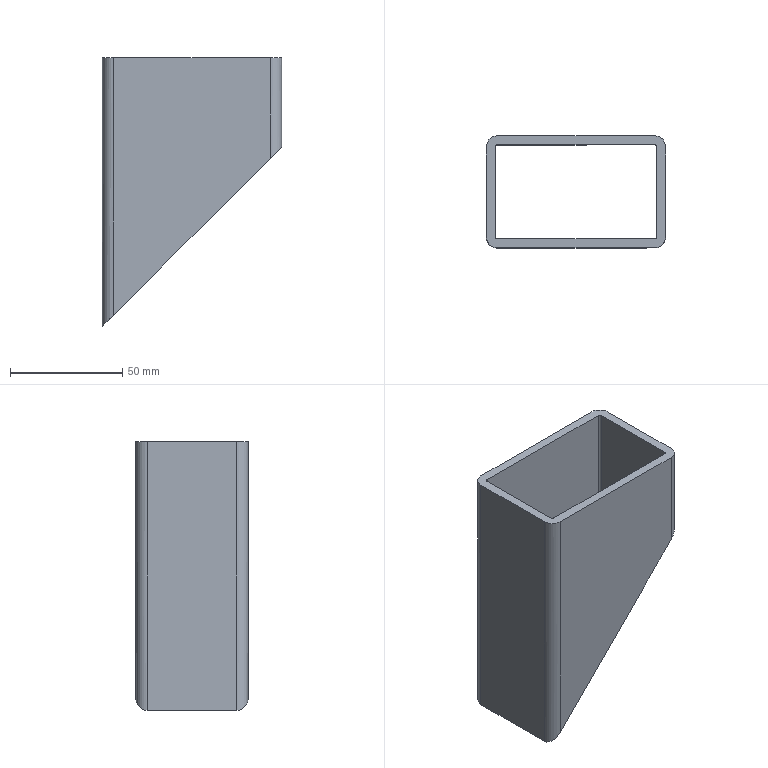Part | SolidWorks | features ICE 3, Extrusion 1, Shell 1 | 1 solid | 18 faces | box 80 x 50 x 120 mm | volume 76432 mm3 | plane 10 | cylinder 8 | commonest cylinder face diameters 2 x4 10 x4
STEP:
#1=CARTESIAN_POINT('',(-40.,20.,120.));
#2=VERTEX_POINT('',#1);
#3=CARTESIAN_POINT('',(-40.,20.,0.));
#4=VERTEX_POINT('',#3);
#5=CARTESIAN_POINT('',(-40.,20.,2200.));
#6=DIRECTION('',(0.,0.,-1.));
#7=VECTOR('',#6,1000.);
#8=LINE('',#5,#7);
#9=EDGE_CURVE('',#2,#4,#8,.T.);
#10=ORIENTED_EDGE('',*,*,#9,.F.);
#11=CARTESIAN_POINT('',(-35.,25.,120.));
#12=VERTEX_POINT('',#11);
#13=CARTESIAN_POINT('',(-35.,20.,120.));
#14=DIRECTION('',(0.,0.,-1.));
#15=DIRECTION('',(-1.,0.,0.));
#16=AXIS2_PLACEMENT_3D('',#13,#14,#15);
#17=CIRCLE('',#16,5.);
#18=EDGE_CURVE('',#2,#12,#17,.T.);
#19=ORIENTED_EDGE('',*,*,#18,.T.);
#20=CARTESIAN_POINT('',(-35.,25.,5.));
#21=VERTEX_POINT('',#20);
#22=CARTESIAN_POINT('',(-35.,25.,2200.));
#23=DIRECTION('',(0.,0.,-1.));
#24=VECTOR('',#23,1000.);
#25=LINE('',#22,#24);
#26=EDGE_CURVE('',#12,#21,#25,.T.);
#27=ORIENTED_EDGE('',*,*,#26,.T.);
#28=CARTESIAN_POINT('',(-35.,25.,5.));
#29=CARTESIAN_POINT('',(-37.929,25.,2.071));
#30=CARTESIAN_POINT('',(-40.,22.929,0.));
#31=CARTESIAN_POINT('',(-40.,20.,0.));
#32=(BOUNDED_CURVE()B_SPLINE_CURVE(3,(#28,#29,#30,#31),.UNSPECIFIED.,.F.,.T.)B_SPLINE_CURVE_WITH_KNOTS((4,4),(4.712,6.283),.UNSPECIFIED.)CURVE()GEOMETRIC_REPRESENTATION_ITEM()RATIONAL_B_SPLINE_CURVE((1.,0.8047,0.8047,1.))REPRESENTATION_ITEM(''));
#33=EDGE_CURVE('',#21,#4,#32,.T.);
#34=ORIENTED_EDGE('',*,*,#33,.T.);
#35=EDGE_LOOP('',(#10,#19,#27,#34));
#36=FACE_OUTER_BOUND('',#35,.T.);
#37=CARTESIAN_POINT('',(-35.,20.,2200.));
#38=DIRECTION('',(0.,0.,-1.));
#39=DIRECTION('',(-1.,0.,0.));
#40=AXIS2_PLACEMENT_3D('',#37,#38,#39);
#41=CYLINDRICAL_SURFACE('',#40,5.);
#42=ADVANCED_FACE('',(#36),#41,.T.);
#43=CARTESIAN_POINT('',(-40.,-20.,120.));
#44=VERTEX_POINT('',#43);
#45=CARTESIAN_POINT('',(-40.,-20.,0.));
#46=VERTEX_POINT('',#45);
#47=CARTESIAN_POINT('',(-40.,-20.,2200.));
#48=DIRECTION('',(0.,0.,-1.));
#49=VECTOR('',#48,1000.);
#50=LINE('',#47,#49);
#51=EDGE_CURVE('',#44,#46,#50,.T.);
#52=ORIENTED_EDGE('',*,*,#51,.F.);
#53=CARTESIAN_POINT('',(-40.,20.,120.));
#54=DIRECTION('',(0.,1.,0.));
#55=VECTOR('',#54,1000.);
#56=LINE('',#53,#55);
#57=EDGE_CURVE('',#44,#2,#56,.T.);
#58=ORIENTED_EDGE('',*,*,#57,.T.);
#59=ORIENTED_EDGE('',*,*,#9,.T.);
#60=CARTESIAN_POINT('',(-40.,20.,0.));
#61=DIRECTION('',(0.,-1.,0.));
#62=VECTOR('',#61,1000.);
#63=LINE('',#60,#62);
#64=EDGE_CURVE('',#4,#46,#63,.T.);
#65=ORIENTED_EDGE('',*,*,#64,.T.);
#66=EDGE_LOOP('',(#52,#58,#59,#65));
#67=FACE_OUTER_BOUND('',#66,.T.);
#68=CARTESIAN_POINT('',(-40.,20.,2200.));
#69=DIRECTION('',(1.,0.,0.));
#70=DIRECTION('',(0.,1.,0.));
#71=AXIS2_PLACEMENT_3D('',#68,#69,#70);
#72=PLANE('',#71);
#73=ADVANCED_FACE('',(#67),#72,.F.);
#74=CARTESIAN_POINT('',(-35.,-25.,120.));
#75=VERTEX_POINT('',#74);
#76=CARTESIAN_POINT('',(-35.,-20.,120.));
#77=DIRECTION('',(0.,0.,1.));
#78=DIRECTION('',(-1.,0.,0.));
#79=AXIS2_PLACEMENT_3D('',#76,#77,#78);
#80=CIRCLE('',#79,5.);
#81=EDGE_CURVE('',#44,#75,#80,.T.);
#82=ORIENTED_EDGE('',*,*,#81,.F.);
#83=ORIENTED_EDGE('',*,*,#51,.T.);
#84=CARTESIAN_POINT('',(-35.,-25.,5.));
#85=VERTEX_POINT('',#84);
#86=CARTESIAN_POINT('',(-35.,-25.,5.));
#87=CARTESIAN_POINT('',(-37.929,-25.,2.071));
#88=CARTESIAN_POINT('',(-40.,-22.929,0.));
#89=CARTESIAN_POINT('',(-40.,-20.,0.));
#90=(BOUNDED_CURVE()B_SPLINE_CURVE(3,(#86,#87,#88,#89),.UNSPECIFIED.,.F.,.F.)B_SPLINE_CURVE_WITH_KNOTS((4,4),(4.712,6.283),.UNSPECIFIED.)CURVE()GEOMETRIC_REPRESENTATION_ITEM()RATIONAL_B_SPLINE_CURVE((1.,0.8047,0.8047,1.))REPRESENTATION_ITEM(''));
#91=EDGE_CURVE('',#85,#46,#90,.T.);
#92=ORIENTED_EDGE('',*,*,#91,.F.);
#93=CARTESIAN_POINT('',(-35.,-25.,2200.));
#94=DIRECTION('',(0.,0.,-1.));
#95=VECTOR('',#94,1000.);
#96=LINE('',#93,#95);
#97=EDGE_CURVE('',#75,#85,#96,.T.);
#98=ORIENTED_EDGE('',*,*,#97,.F.);
#99=EDGE_LOOP('',(#82,#83,#92,#98));
#100=FACE_OUTER_BOUND('',#99,.T.);
#101=CARTESIAN_POINT('',(-35.,-20.,2200.));
#102=DIRECTION('',(0.,0.,-1.));
#103=DIRECTION('',(-1.,0.,0.));
#104=AXIS2_PLACEMENT_3D('',#101,#102,#103);
#105=CYLINDRICAL_SURFACE('',#104,5.);
#106=ADVANCED_FACE('',(#100),#105,.T.);
#107=CARTESIAN_POINT('',(35.,-25.,120.));
#108=VERTEX_POINT('',#107);
#109=CARTESIAN_POINT('',(1017.702,-25.,120.));
#110=DIRECTION('',(1.,0.,0.));
#111=VECTOR('',#110,1000.);
#112=LINE('',#109,#111);
#113=EDGE_CURVE('',#75,#108,#112,.T.);
#114=ORIENTED_EDGE('',*,*,#113,.F.);
#115=ORIENTED_EDGE('',*,*,#97,.T.);
#116=CARTESIAN_POINT('',(35.,-25.,75.));
#117=VERTEX_POINT('',#116);
#118=CARTESIAN_POINT('',(-40.,-25.,0.));
#119=DIRECTION('',(-0.7071,0.,-0.7071));
#120=VECTOR('',#119,1000.);
#121=LINE('',#118,#120);
#122=EDGE_CURVE('',#117,#85,#121,.T.);
#123=ORIENTED_EDGE('',*,*,#122,.F.);
#124=CARTESIAN_POINT('',(35.,-25.,2200.));
#125=DIRECTION('',(0.,0.,-1.));
#126=VECTOR('',#125,1000.);
#127=LINE('',#124,#126);
#128=EDGE_CURVE('',#108,#117,#127,.T.);
#129=ORIENTED_EDGE('',*,*,#128,.F.);
#130=EDGE_LOOP('',(#114,#115,#123,#129));
#131=FACE_OUTER_BOUND('',#130,.T.);
#132=CARTESIAN_POINT('',(35.,-25.,2200.));
#133=DIRECTION('',(0.,-1.,0.));
#134=DIRECTION('',(1.,0.,0.));
#135=AXIS2_PLACEMENT_3D('',#132,#133,#134);
#136=PLANE('',#135);
#137=ADVANCED_FACE('',(#131),#136,.T.);
#138=CARTESIAN_POINT('',(40.,-20.,120.));
#139=VERTEX_POINT('',#138);
#140=CARTESIAN_POINT('',(35.,-20.,120.));
#141=DIRECTION('',(0.,0.,1.));
#142=DIRECTION('',(-1.,0.,0.));
#143=AXIS2_PLACEMENT_3D('',#140,#141,#142);
#144=CIRCLE('',#143,5.);
#145=EDGE_CURVE('',#108,#139,#144,.T.);
#146=ORIENTED_EDGE('',*,*,#145,.F.);
#147=ORIENTED_EDGE('',*,*,#128,.T.);
#148=CARTESIAN_POINT('',(40.,-20.,80.));
#149=VERTEX_POINT('',#148);
#150=CARTESIAN_POINT('',(40.,-20.,80.));
#151=CARTESIAN_POINT('',(40.,-22.929,80.));
#152=CARTESIAN_POINT('',(37.929,-25.,77.929));
#153=CARTESIAN_POINT('',(35.,-25.,75.));
#154=(BOUNDED_CURVE()B_SPLINE_CURVE(3,(#150,#151,#152,#153),.UNSPECIFIED.,.F.,.F.)B_SPLINE_CURVE_WITH_KNOTS((4,4),(3.142,4.712),.UNSPECIFIED.)CURVE()GEOMETRIC_REPRESENTATION_ITEM()RATIONAL_B_SPLINE_CURVE((1.,0.8047,0.8047,1.))REPRESENTATION_ITEM(''));
#155=EDGE_CURVE('',#149,#117,#154,.T.);
#156=ORIENTED_EDGE('',*,*,#155,.F.);
#157=CARTESIAN_POINT('',(40.,-20.,2200.));
#158=DIRECTION('',(0.,0.,-1.));
#159=VECTOR('',#158,1000.);
#160=LINE('',#157,#159);
#161=EDGE_CURVE('',#139,#149,#160,.T.);
#162=ORIENTED_EDGE('',*,*,#161,.F.);
#163=EDGE_LOOP('',(#146,#147,#156,#162));
#164=FACE_OUTER_BOUND('',#163,.T.);
#165=CARTESIAN_POINT('',(35.,-20.,2200.));
#166=DIRECTION('',(0.,0.,-1.));
#167=DIRECTION('',(-1.,0.,0.));
#168=AXIS2_PLACEMENT_3D('',#165,#166,#167);
#169=CYLINDRICAL_SURFACE('',#168,5.);
#170=ADVANCED_FACE('',(#164),#169,.T.);
#171=CARTESIAN_POINT('',(40.,20.,120.));
#172=VERTEX_POINT('',#171);
#173=CARTESIAN_POINT('',(40.,20.,120.));
#174=DIRECTION('',(0.,1.,0.));
#175=VECTOR('',#174,1000.);
#176=LINE('',#173,#175);
#177=EDGE_CURVE('',#139,#172,#176,.T.);
#178=ORIENTED_EDGE('',*,*,#177,.F.);
#179=ORIENTED_EDGE('',*,*,#161,.T.);
#180=CARTESIAN_POINT('',(40.,20.,80.));
#181=VERTEX_POINT('',#180);
#182=CARTESIAN_POINT('',(40.,1975.,80.));
#183=DIRECTION('',(0.,-1.,0.));
#184=VECTOR('',#183,1000.);
#185=LINE('',#182,#184);
#186=EDGE_CURVE('',#181,#149,#185,.T.);
#187=ORIENTED_EDGE('',*,*,#186,.F.);
#188=CARTESIAN_POINT('',(40.,20.,2200.));
#189=DIRECTION('',(0.,0.,-1.));
#190=VECTOR('',#189,1000.);
#191=LINE('',#188,#190);
#192=EDGE_CURVE('',#172,#181,#191,.T.);
#193=ORIENTED_EDGE('',*,*,#192,.F.);
#194=EDGE_LOOP('',(#178,#179,#187,#193));
#195=FACE_OUTER_BOUND('',#194,.T.);
#196=CARTESIAN_POINT('',(40.,20.,2200.));
#197=DIRECTION('',(1.,0.,0.));
#198=DIRECTION('',(0.,1.,0.));
#199=AXIS2_PLACEMENT_3D('',#196,#197,#198);
#200=PLANE('',#199);
#201=ADVANCED_FACE('',(#195),#200,.T.);
#202=CARTESIAN_POINT('',(35.,25.,120.));
#203=VERTEX_POINT('',#202);
#204=CARTESIAN_POINT('',(35.,20.,120.));
#205=DIRECTION('',(0.,0.,1.));
#206=DIRECTION('',(-1.,0.,0.));
#207=AXIS2_PLACEMENT_3D('',#204,#205,#206);
#208=CIRCLE('',#207,5.);
#209=EDGE_CURVE('',#172,#203,#208,.T.);
#210=ORIENTED_EDGE('',*,*,#209,.F.);
#211=ORIENTED_EDGE('',*,*,#192,.T.);
#212=CARTESIAN_POINT('',(35.,25.,75.));
#213=VERTEX_POINT('',#212);
#214=CARTESIAN_POINT('',(35.,25.,75.));
#215=CARTESIAN_POINT('',(37.929,25.,77.929));
#216=CARTESIAN_POINT('',(40.,22.929,80.));
#217=CARTESIAN_POINT('',(40.,20.,80.));
#218=(BOUNDED_CURVE()B_SPLINE_CURVE(3,(#214,#215,#216,#217),.UNSPECIFIED.,.F.,.F.)B_SPLINE_CURVE_WITH_KNOTS((4,4),(1.571,3.142),.UNSPECIFIED.)CURVE()GEOMETRIC_REPRESENTATION_ITEM()RATIONAL_B_SPLINE_CURVE((1.,0.8047,0.8047,1.))REPRESENTATION_ITEM(''));
#219=EDGE_CURVE('',#213,#181,#218,.T.);
#220=ORIENTED_EDGE('',*,*,#219,.F.);
#221=CARTESIAN_POINT('',(35.,25.,2200.));
#222=DIRECTION('',(0.,0.,-1.));
#223=VECTOR('',#222,1000.);
#224=LINE('',#221,#223);
#225=EDGE_CURVE('',#203,#213,#224,.T.);
#226=ORIENTED_EDGE('',*,*,#225,.F.);
#227=EDGE_LOOP('',(#210,#211,#220,#226));
#228=FACE_OUTER_BOUND('',#227,.T.);
#229=CARTESIAN_POINT('',(35.,20.,2200.));
#230=DIRECTION('',(0.,0.,-1.));
#231=DIRECTION('',(-1.,0.,0.));
#232=AXIS2_PLACEMENT_3D('',#229,#230,#231);
#233=CYLINDRICAL_SURFACE('',#232,5.);
#234=ADVANCED_FACE('',(#228),#233,.T.);
#235=ORIENTED_EDGE('',*,*,#26,.F.);
#236=CARTESIAN_POINT('',(35.,25.,120.));
#237=DIRECTION('',(1.,0.,0.));
#238=VECTOR('',#237,1000.);
#239=LINE('',#236,#238);
#240=EDGE_CURVE('',#12,#203,#239,.T.);
#241=ORIENTED_EDGE('',*,*,#240,.T.);
#242=ORIENTED_EDGE('',*,*,#225,.T.);
#243=CARTESIAN_POINT('',(1097.5,25.,1137.5));
#244=DIRECTION('',(-0.7071,0.,-0.7071));
#245=VECTOR('',#244,1000.);
#246=LINE('',#243,#245);
#247=EDGE_CURVE('',#213,#21,#246,.T.);
#248=ORIENTED_EDGE('',*,*,#247,.T.);
#249=EDGE_LOOP('',(#235,#241,#242,#248));
#250=FACE_OUTER_BOUND('',#249,.T.);
#251=CARTESIAN_POINT('',(35.,25.,2200.));
#252=DIRECTION('',(0.,-1.,0.));
#253=DIRECTION('',(1.,0.,0.));
#254=AXIS2_PLACEMENT_3D('',#251,#252,#253);
#255=PLANE('',#254);
#256=ADVANCED_FACE('',(#250),#255,.F.);
#257=CARTESIAN_POINT('',(-36.,20.,120.));
#258=VERTEX_POINT('',#257);
#259=CARTESIAN_POINT('',(-35.,21.,120.));
#260=VERTEX_POINT('',#259);
#261=CARTESIAN_POINT('',(-35.,20.,120.));
#262=DIRECTION('',(0.,0.,-1.));
#263=DIRECTION('',(-1.,0.,0.));
#264=AXIS2_PLACEMENT_3D('',#261,#262,#263);
#265=CIRCLE('',#264,1.);
#266=EDGE_CURVE('',#258,#260,#265,.T.);
#267=ORIENTED_EDGE('',*,*,#266,.F.);
#268=CARTESIAN_POINT('',(-36.,20.,4.));
#269=VERTEX_POINT('',#268);
#270=CARTESIAN_POINT('',(-36.,20.,2200.));
#271=DIRECTION('',(0.,0.,-1.));
#272=VECTOR('',#271,1000.);
#273=LINE('',#270,#272);
#274=EDGE_CURVE('',#258,#269,#273,.T.);
#275=ORIENTED_EDGE('',*,*,#274,.T.);
#276=CARTESIAN_POINT('',(-35.,21.,5.));
#277=VERTEX_POINT('',#276);
#278=CARTESIAN_POINT('',(-35.,21.,5.));
#279=CARTESIAN_POINT('',(-35.586,21.,4.414));
#280=CARTESIAN_POINT('',(-36.,20.586,4.));
#281=CARTESIAN_POINT('',(-36.,20.,4.));
#282=(BOUNDED_CURVE()B_SPLINE_CURVE(3,(#278,#279,#280,#281),.UNSPECIFIED.,.F.,.T.)B_SPLINE_CURVE_WITH_KNOTS((4,4),(4.712,6.283),.UNSPECIFIED.)CURVE()GEOMETRIC_REPRESENTATION_ITEM()RATIONAL_B_SPLINE_CURVE((1.,0.8047,0.8047,1.))REPRESENTATION_ITEM(''));
#283=EDGE_CURVE('',#277,#269,#282,.T.);
#284=ORIENTED_EDGE('',*,*,#283,.F.);
#285=CARTESIAN_POINT('',(-35.,21.,2200.));
#286=DIRECTION('',(0.,0.,-1.));
#287=VECTOR('',#286,1000.);
#288=LINE('',#285,#287);
#289=EDGE_CURVE('',#260,#277,#288,.T.);
#290=ORIENTED_EDGE('',*,*,#289,.F.);
#291=EDGE_LOOP('',(#267,#275,#284,#290));
#292=FACE_OUTER_BOUND('',#291,.T.);
#293=CARTESIAN_POINT('',(-35.,20.,2200.));
#294=DIRECTION('',(0.,0.,-1.));
#295=DIRECTION('',(-1.,0.,0.));
#296=AXIS2_PLACEMENT_3D('',#293,#294,#295);
#297=CYLINDRICAL_SURFACE('',#296,1.);
#298=ADVANCED_FACE('',(#292),#297,.F.);
#299=CARTESIAN_POINT('',(-36.,-20.,120.));
#300=VERTEX_POINT('',#299);
#301=CARTESIAN_POINT('',(-36.,20.,120.));
#302=DIRECTION('',(0.,1.,0.));
#303=VECTOR('',#302,1000.);
#304=LINE('',#301,#303);
#305=EDGE_CURVE('',#300,#258,#304,.T.);
#306=ORIENTED_EDGE('',*,*,#305,.F.);
#307=CARTESIAN_POINT('',(-36.,-20.,4.));
#308=VERTEX_POINT('',#307);
#309=CARTESIAN_POINT('',(-36.,-20.,2200.));
#310=DIRECTION('',(0.,0.,-1.));
#311=VECTOR('',#310,1000.);
#312=LINE('',#309,#311);
#313=EDGE_CURVE('',#300,#308,#312,.T.);
#314=ORIENTED_EDGE('',*,*,#313,.T.);
#315=CARTESIAN_POINT('',(-36.,20.,4.));
#316=DIRECTION('',(0.,-1.,0.));
#317=VECTOR('',#316,1000.);
#318=LINE('',#315,#317);
#319=EDGE_CURVE('',#269,#308,#318,.T.);
#320=ORIENTED_EDGE('',*,*,#319,.F.);
#321=ORIENTED_EDGE('',*,*,#274,.F.);
#322=EDGE_LOOP('',(#306,#314,#320,#321));
#323=FACE_OUTER_BOUND('',#322,.T.);
#324=CARTESIAN_POINT('',(-36.,20.,2200.));
#325=DIRECTION('',(1.,0.,0.));
#326=DIRECTION('',(0.,1.,0.));
#327=AXIS2_PLACEMENT_3D('',#324,#325,#326);
#328=PLANE('',#327);
#329=ADVANCED_FACE('',(#323),#328,.T.);
#330=ORIENTED_EDGE('',*,*,#313,.F.);
#331=CARTESIAN_POINT('',(-35.,-21.,120.));
#332=VERTEX_POINT('',#331);
#333=CARTESIAN_POINT('',(-35.,-20.,120.));
#334=DIRECTION('',(0.,0.,1.));
#335=DIRECTION('',(-1.,0.,0.));
#336=AXIS2_PLACEMENT_3D('',#333,#334,#335);
#337=CIRCLE('',#336,1.);
#338=EDGE_CURVE('',#300,#332,#337,.T.);
#339=ORIENTED_EDGE('',*,*,#338,.T.);
#340=CARTESIAN_POINT('',(-35.,-21.,5.));
#341=VERTEX_POINT('',#340);
#342=CARTESIAN_POINT('',(-35.,-21.,2200.));
#343=DIRECTION('',(0.,0.,-1.));
#344=VECTOR('',#343,1000.);
#345=LINE('',#342,#344);
#346=EDGE_CURVE('',#332,#341,#345,.T.);
#347=ORIENTED_EDGE('',*,*,#346,.T.);
#348=CARTESIAN_POINT('',(-35.,-21.,5.));
#349=CARTESIAN_POINT('',(-35.586,-21.,4.414));
#350=CARTESIAN_POINT('',(-36.,-20.586,4.));
#351=CARTESIAN_POINT('',(-36.,-20.,4.));
#352=(BOUNDED_CURVE()B_SPLINE_CURVE(3,(#348,#349,#350,#351),.UNSPECIFIED.,.F.,.F.)B_SPLINE_CURVE_WITH_KNOTS((4,4),(4.712,6.283),.UNSPECIFIED.)CURVE()GEOMETRIC_REPRESENTATION_ITEM()RATIONAL_B_SPLINE_CURVE((1.,0.8047,0.8047,1.))REPRESENTATION_ITEM(''));
#353=EDGE_CURVE('',#341,#308,#352,.T.);
#354=ORIENTED_EDGE('',*,*,#353,.T.);
#355=EDGE_LOOP('',(#330,#339,#347,#354));
#356=FACE_OUTER_BOUND('',#355,.T.);
#357=CARTESIAN_POINT('',(-35.,-20.,2200.));
#358=DIRECTION('',(0.,0.,-1.));
#359=DIRECTION('',(-1.,0.,0.));
#360=AXIS2_PLACEMENT_3D('',#357,#358,#359);
#361=CYLINDRICAL_SURFACE('',#360,1.);
#362=ADVANCED_FACE('',(#356),#361,.F.);
#363=ORIENTED_EDGE('',*,*,#346,.F.);
#364=CARTESIAN_POINT('',(35.,-21.,120.));
#365=VERTEX_POINT('',#364);
#366=CARTESIAN_POINT('',(35.,-21.,120.));
#367=DIRECTION('',(1.,0.,0.));
#368=VECTOR('',#367,1000.);
#369=LINE('',#366,#368);
#370=EDGE_CURVE('',#332,#365,#369,.T.);
#371=ORIENTED_EDGE('',*,*,#370,.T.);
#372=CARTESIAN_POINT('',(35.,-21.,75.));
#373=VERTEX_POINT('',#372);
#374=CARTESIAN_POINT('',(35.,-21.,2200.));
#375=DIRECTION('',(0.,0.,-1.));
#376=VECTOR('',#375,1000.);
#377=LINE('',#374,#376);
#378=EDGE_CURVE('',#365,#373,#377,.T.);
#379=ORIENTED_EDGE('',*,*,#378,.T.);
#380=CARTESIAN_POINT('',(1097.5,-21.,1137.5));
#381=DIRECTION('',(-0.7071,0.,-0.7071));
#382=VECTOR('',#381,1000.);
#383=LINE('',#380,#382);
#384=EDGE_CURVE('',#373,#341,#383,.T.);
#385=ORIENTED_EDGE('',*,*,#384,.T.);
#386=EDGE_LOOP('',(#363,#371,#379,#385));
#387=FACE_OUTER_BOUND('',#386,.T.);
#388=CARTESIAN_POINT('',(35.,-21.,2200.));
#389=DIRECTION('',(0.,-1.,0.));
#390=DIRECTION('',(1.,0.,0.));
#391=AXIS2_PLACEMENT_3D('',#388,#389,#390);
#392=PLANE('',#391);
#393=ADVANCED_FACE('',(#387),#392,.F.);
#394=ORIENTED_EDGE('',*,*,#378,.F.);
#395=CARTESIAN_POINT('',(36.,-20.,120.));
#396=VERTEX_POINT('',#395);
#397=CARTESIAN_POINT('',(35.,-20.,120.));
#398=DIRECTION('',(0.,0.,1.));
#399=DIRECTION('',(-1.,0.,0.));
#400=AXIS2_PLACEMENT_3D('',#397,#398,#399);
#401=CIRCLE('',#400,1.);
#402=EDGE_CURVE('',#365,#396,#401,.T.);
#403=ORIENTED_EDGE('',*,*,#402,.T.);
#404=CARTESIAN_POINT('',(36.,-20.,76.));
#405=VERTEX_POINT('',#404);
#406=CARTESIAN_POINT('',(36.,-20.,2200.));
#407=DIRECTION('',(0.,0.,-1.));
#408=VECTOR('',#407,1000.);
#409=LINE('',#406,#408);
#410=EDGE_CURVE('',#396,#405,#409,.T.);
#411=ORIENTED_EDGE('',*,*,#410,.T.);
#412=CARTESIAN_POINT('',(36.,-20.,76.));
#413=CARTESIAN_POINT('',(36.,-20.586,76.));
#414=CARTESIAN_POINT('',(35.586,-21.,75.586));
#415=CARTESIAN_POINT('',(35.,-21.,75.));
#416=(BOUNDED_CURVE()B_SPLINE_CURVE(3,(#412,#413,#414,#415),.UNSPECIFIED.,.F.,.F.)B_SPLINE_CURVE_WITH_KNOTS((4,4),(3.142,4.712),.UNSPECIFIED.)CURVE()GEOMETRIC_REPRESENTATION_ITEM()RATIONAL_B_SPLINE_CURVE((1.,0.8047,0.8047,1.))REPRESENTATION_ITEM(''));
#417=EDGE_CURVE('',#405,#373,#416,.T.);
#418=ORIENTED_EDGE('',*,*,#417,.T.);
#419=EDGE_LOOP('',(#394,#403,#411,#418));
#420=FACE_OUTER_BOUND('',#419,.T.);
#421=CARTESIAN_POINT('',(35.,-20.,2200.));
#422=DIRECTION('',(0.,0.,-1.));
#423=DIRECTION('',(-1.,0.,0.));
#424=AXIS2_PLACEMENT_3D('',#421,#422,#423);
#425=CYLINDRICAL_SURFACE('',#424,1.);
#426=ADVANCED_FACE('',(#420),#425,.F.);
#427=ORIENTED_EDGE('',*,*,#410,.F.);
#428=CARTESIAN_POINT('',(36.,20.,120.));
#429=VERTEX_POINT('',#428);
#430=CARTESIAN_POINT('',(36.,20.,120.));
#431=DIRECTION('',(0.,1.,0.));
#432=VECTOR('',#431,1000.);
#433=LINE('',#430,#432);
#434=EDGE_CURVE('',#396,#429,#433,.T.);
#435=ORIENTED_EDGE('',*,*,#434,.T.);
#436=CARTESIAN_POINT('',(36.,20.,76.));
#437=VERTEX_POINT('',#436);
#438=CARTESIAN_POINT('',(36.,20.,2200.));
#439=DIRECTION('',(0.,0.,-1.));
#440=VECTOR('',#439,1000.);
#441=LINE('',#438,#440);
#442=EDGE_CURVE('',#429,#437,#441,.T.);
#443=ORIENTED_EDGE('',*,*,#442,.T.);
#444=CARTESIAN_POINT('',(36.,20.,76.));
#445=DIRECTION('',(0.,-1.,0.));
#446=VECTOR('',#445,1000.);
#447=LINE('',#444,#446);
#448=EDGE_CURVE('',#437,#405,#447,.T.);
#449=ORIENTED_EDGE('',*,*,#448,.T.);
#450=EDGE_LOOP('',(#427,#435,#443,#449));
#451=FACE_OUTER_BOUND('',#450,.T.);
#452=CARTESIAN_POINT('',(36.,20.,2200.));
#453=DIRECTION('',(1.,0.,0.));
#454=DIRECTION('',(0.,1.,0.));
#455=AXIS2_PLACEMENT_3D('',#452,#453,#454);
#456=PLANE('',#455);
#457=ADVANCED_FACE('',(#451),#456,.F.);
#458=ORIENTED_EDGE('',*,*,#442,.F.);
#459=CARTESIAN_POINT('',(35.,21.,120.));
#460=VERTEX_POINT('',#459);
#461=CARTESIAN_POINT('',(35.,20.,120.));
#462=DIRECTION('',(0.,0.,1.));
#463=DIRECTION('',(-1.,0.,0.));
#464=AXIS2_PLACEMENT_3D('',#461,#462,#463);
#465=CIRCLE('',#464,1.);
#466=EDGE_CURVE('',#429,#460,#465,.T.);
#467=ORIENTED_EDGE('',*,*,#466,.T.);
#468=CARTESIAN_POINT('',(35.,21.,75.));
#469=VERTEX_POINT('',#468);
#470=CARTESIAN_POINT('',(35.,21.,2200.));
#471=DIRECTION('',(0.,0.,-1.));
#472=VECTOR('',#471,1000.);
#473=LINE('',#470,#472);
#474=EDGE_CURVE('',#460,#469,#473,.T.);
#475=ORIENTED_EDGE('',*,*,#474,.T.);
#476=CARTESIAN_POINT('',(35.,21.,75.));
#477=CARTESIAN_POINT('',(35.586,21.,75.586));
#478=CARTESIAN_POINT('',(36.,20.586,76.));
#479=CARTESIAN_POINT('',(36.,20.,76.));
#480=(BOUNDED_CURVE()B_SPLINE_CURVE(3,(#476,#477,#478,#479),.UNSPECIFIED.,.F.,.F.)B_SPLINE_CURVE_WITH_KNOTS((4,4),(1.571,3.142),.UNSPECIFIED.)CURVE()GEOMETRIC_REPRESENTATION_ITEM()RATIONAL_B_SPLINE_CURVE((1.,0.8047,0.8047,1.))REPRESENTATION_ITEM(''));
#481=EDGE_CURVE('',#469,#437,#480,.T.);
#482=ORIENTED_EDGE('',*,*,#481,.T.);
#483=EDGE_LOOP('',(#458,#467,#475,#482));
#484=FACE_OUTER_BOUND('',#483,.T.);
#485=CARTESIAN_POINT('',(35.,20.,2200.));
#486=DIRECTION('',(0.,0.,-1.));
#487=DIRECTION('',(-1.,0.,0.));
#488=AXIS2_PLACEMENT_3D('',#485,#486,#487);
#489=CYLINDRICAL_SURFACE('',#488,1.);
#490=ADVANCED_FACE('',(#484),#489,.F.);
#491=CARTESIAN_POINT('',(35.,21.,120.));
#492=DIRECTION('',(1.,0.,0.));
#493=VECTOR('',#492,1000.);
#494=LINE('',#491,#493);
#495=EDGE_CURVE('',#260,#460,#494,.T.);
#496=ORIENTED_EDGE('',*,*,#495,.F.);
#497=ORIENTED_EDGE('',*,*,#289,.T.);
#498=CARTESIAN_POINT('',(1097.5,21.,1137.5));
#499=DIRECTION('',(-0.7071,0.,-0.7071));
#500=VECTOR('',#499,1000.);
#501=LINE('',#498,#500);
#502=EDGE_CURVE('',#469,#277,#501,.T.);
#503=ORIENTED_EDGE('',*,*,#502,.F.);
#504=ORIENTED_EDGE('',*,*,#474,.F.);
#505=EDGE_LOOP('',(#496,#497,#503,#504));
#506=FACE_OUTER_BOUND('',#505,.T.);
#507=CARTESIAN_POINT('',(35.,21.,2200.));
#508=DIRECTION('',(0.,-1.,0.));
#509=DIRECTION('',(1.,0.,0.));
#510=AXIS2_PLACEMENT_3D('',#507,#508,#509);
#511=PLANE('',#510);
#512=ADVANCED_FACE('',(#506),#511,.T.);
#513=ORIENTED_EDGE('',*,*,#91,.T.);
#514=ORIENTED_EDGE('',*,*,#64,.F.);
#515=ORIENTED_EDGE('',*,*,#33,.F.);
#516=ORIENTED_EDGE('',*,*,#247,.F.);
#517=ORIENTED_EDGE('',*,*,#219,.T.);
#518=ORIENTED_EDGE('',*,*,#186,.T.);
#519=ORIENTED_EDGE('',*,*,#155,.T.);
#520=ORIENTED_EDGE('',*,*,#122,.T.);
#521=EDGE_LOOP('',(#513,#514,#515,#516,#517,#518,#519,#520));
#522=FACE_OUTER_BOUND('',#521,.T.);
#523=ORIENTED_EDGE('',*,*,#283,.T.);
#524=ORIENTED_EDGE('',*,*,#319,.T.);
#525=ORIENTED_EDGE('',*,*,#353,.F.);
#526=ORIENTED_EDGE('',*,*,#384,.F.);
#527=ORIENTED_EDGE('',*,*,#417,.F.);
#528=ORIENTED_EDGE('',*,*,#448,.F.);
#529=ORIENTED_EDGE('',*,*,#481,.F.);
#530=ORIENTED_EDGE('',*,*,#502,.T.);
#531=EDGE_LOOP('',(#523,#524,#525,#526,#527,#528,#529,#530));
#532=FACE_BOUND('',#531,.T.);
#533=CARTESIAN_POINT('',(-40.,1975.,0.));
#534=DIRECTION('',(-0.7071,0.,0.7071));
#535=DIRECTION('',(0.7071,0.,0.7071));
#536=AXIS2_PLACEMENT_3D('',#533,#534,#535);
#537=PLANE('',#536);
#538=ADVANCED_FACE('',(#522,#532),#537,.F.);
#539=ORIENTED_EDGE('',*,*,#81,.T.);
#540=ORIENTED_EDGE('',*,*,#113,.T.);
#541=ORIENTED_EDGE('',*,*,#145,.T.);
#542=ORIENTED_EDGE('',*,*,#177,.T.);
#543=ORIENTED_EDGE('',*,*,#209,.T.);
#544=ORIENTED_EDGE('',*,*,#240,.F.);
#545=ORIENTED_EDGE('',*,*,#18,.F.);
#546=ORIENTED_EDGE('',*,*,#57,.F.);
#547=EDGE_LOOP('',(#539,#540,#541,#542,#543,#544,#545,#546));
#548=FACE_OUTER_BOUND('',#547,.T.);
#549=ORIENTED_EDGE('',*,*,#266,.T.);
#550=ORIENTED_EDGE('',*,*,#495,.T.);
#551=ORIENTED_EDGE('',*,*,#466,.F.);
#552=ORIENTED_EDGE('',*,*,#434,.F.);
#553=ORIENTED_EDGE('',*,*,#402,.F.);
#554=ORIENTED_EDGE('',*,*,#370,.F.);
#555=ORIENTED_EDGE('',*,*,#338,.F.);
#556=ORIENTED_EDGE('',*,*,#305,.T.);
#557=EDGE_LOOP('',(#549,#550,#551,#552,#553,#554,#555,#556));
#558=FACE_BOUND('',#557,.T.);
#559=CARTESIAN_POINT('',(1017.702,1975.,120.));
#560=DIRECTION('',(0.,0.,-1.));
#561=DIRECTION('',(-1.,0.,0.));
#562=AXIS2_PLACEMENT_3D('',#559,#560,#561);
#563=PLANE('',#562);
#564=ADVANCED_FACE('',(#548,#558),#563,.F.);
#565=CLOSED_SHELL('',(#42,#73,#106,#137,#170,#201,#234,#256,#298,#329,#362,#393,#426,#457,#490,#512,#538,#564));
#566=MANIFOLD_SOLID_BREP('',#565);
#567=CARTESIAN_POINT('',(0.,0.,0.));
#568=DIRECTION('',(0.,0.,1.));
#569=DIRECTION('',(1.,0.,0.));
#570=AXIS2_PLACEMENT_3D('',#567,#568,#569);
#571=(LENGTH_UNIT()NAMED_UNIT(*)SI_UNIT(.MILLI.,.METRE.));
#572=UNCERTAINTY_MEASURE_WITH_UNIT(LENGTH_MEASURE(0.00001),#571,'','');
#573=(NAMED_UNIT(*)PLANE_ANGLE_UNIT()SI_UNIT($,.RADIAN.));
#574=(NAMED_UNIT(*)SI_UNIT($,.STERADIAN.)SOLID_ANGLE_UNIT());
#575=(GEOMETRIC_REPRESENTATION_CONTEXT(3)GLOBAL_UNCERTAINTY_ASSIGNED_CONTEXT((#572))GLOBAL_UNIT_ASSIGNED_CONTEXT((#571,#573,#574))REPRESENTATION_CONTEXT('',''));
#576=ADVANCED_BREP_SHAPE_REPRESENTATION('',(#566,#570),#575);